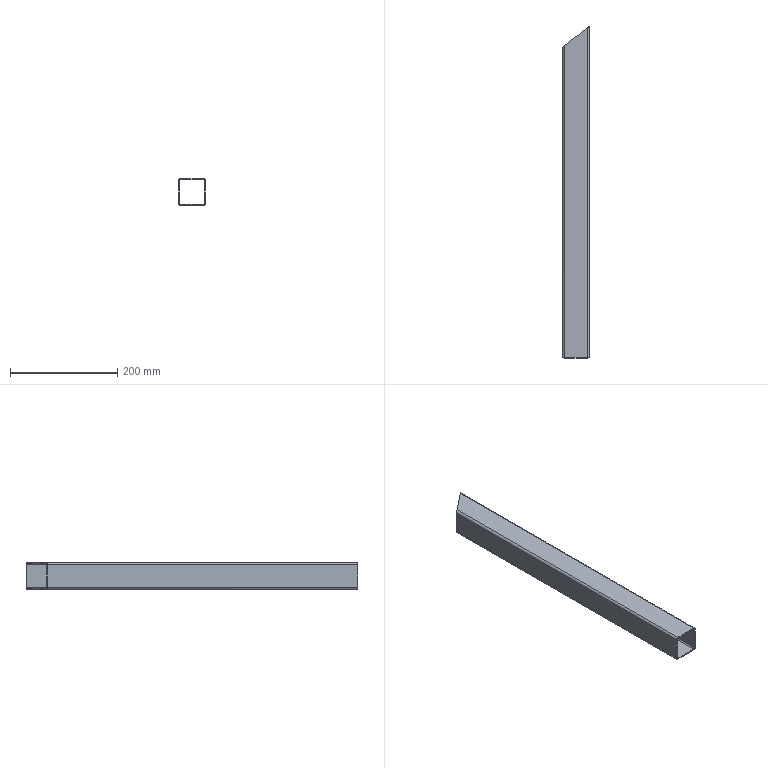Part | STEP file | Microwave Drying Flat Conveyor-CN2500x400-105-101_Default<Machining blank> | 1 solid | 18 faces | box 50 x 620 x 50 mm | volume 224219 mm3 | plane 10 | cylinder 8 | commonest cylinder face diameters 4 x4 8 x4
STEP:
#1=CARTESIAN_POINT('',(501.,0.,21.));
#2=VERTEX_POINT('',#1);
#3=CARTESIAN_POINT('',(501.,620.,21.));
#4=VERTEX_POINT('',#3);
#5=CARTESIAN_POINT('',(501.,0.,21.));
#6=DIRECTION('',(0.,1.,0.));
#7=VECTOR('',#6,1000.);
#8=LINE('',#5,#7);
#9=EDGE_CURVE('',#2,#4,#8,.T.);
#10=ORIENTED_EDGE('',*,*,#9,.T.);
#11=CARTESIAN_POINT('',(497.,616.8,25.));
#12=VERTEX_POINT('',#11);
#13=CARTESIAN_POINT('',(501.,620.,21.));
#14=CARTESIAN_POINT('',(501.,620.,23.343));
#15=CARTESIAN_POINT('',(499.343,618.675,25.));
#16=CARTESIAN_POINT('',(497.,616.8,25.));
#17=(BOUNDED_CURVE()B_SPLINE_CURVE(3,(#13,#14,#15,#16),.UNSPECIFIED.,.F.,.T.)B_SPLINE_CURVE_WITH_KNOTS((4,4),(0.,1.571),.UNSPECIFIED.)CURVE()GEOMETRIC_REPRESENTATION_ITEM()RATIONAL_B_SPLINE_CURVE((1.,0.8047,0.8047,1.))REPRESENTATION_ITEM(''));
#18=EDGE_CURVE('',#4,#12,#17,.T.);
#19=ORIENTED_EDGE('',*,*,#18,.T.);
#20=CARTESIAN_POINT('',(497.,0.,25.));
#21=VERTEX_POINT('',#20);
#22=CARTESIAN_POINT('',(497.,0.,25.));
#23=DIRECTION('',(0.,1.,0.));
#24=VECTOR('',#23,1000.);
#25=LINE('',#22,#24);
#26=EDGE_CURVE('',#21,#12,#25,.T.);
#27=ORIENTED_EDGE('',*,*,#26,.F.);
#28=CARTESIAN_POINT('',(497.,0.,21.));
#29=DIRECTION('',(0.,-1.,0.));
#30=DIRECTION('',(1.,0.,0.));
#31=AXIS2_PLACEMENT_3D('',#28,#29,#30);
#32=CIRCLE('',#31,4.);
#33=EDGE_CURVE('',#2,#21,#32,.T.);
#34=ORIENTED_EDGE('',*,*,#33,.F.);
#35=EDGE_LOOP('',(#10,#19,#27,#34));
#36=FACE_OUTER_BOUND('',#35,.T.);
#37=CARTESIAN_POINT('',(497.,0.,21.));
#38=DIRECTION('',(0.,1.,0.));
#39=DIRECTION('',(-1.,0.,0.));
#40=AXIS2_PLACEMENT_3D('',#37,#38,#39);
#41=CYLINDRICAL_SURFACE('',#40,4.);
#42=ADVANCED_FACE('',(#36),#41,.T.);
#43=ORIENTED_EDGE('',*,*,#26,.T.);
#44=CARTESIAN_POINT('',(455.,583.2,25.));
#45=VERTEX_POINT('',#44);
#46=CARTESIAN_POINT('',(501.,620.,25.));
#47=DIRECTION('',(0.7809,0.6247,0.));
#48=VECTOR('',#47,1000.);
#49=LINE('',#46,#48);
#50=EDGE_CURVE('',#45,#12,#49,.T.);
#51=ORIENTED_EDGE('',*,*,#50,.F.);
#52=CARTESIAN_POINT('',(455.,0.,25.));
#53=VERTEX_POINT('',#52);
#54=CARTESIAN_POINT('',(455.,0.,25.));
#55=DIRECTION('',(0.,1.,0.));
#56=VECTOR('',#55,1000.);
#57=LINE('',#54,#56);
#58=EDGE_CURVE('',#53,#45,#57,.T.);
#59=ORIENTED_EDGE('',*,*,#58,.F.);
#60=CARTESIAN_POINT('',(497.,0.,25.));
#61=DIRECTION('',(-1.,0.,0.));
#62=VECTOR('',#61,1000.);
#63=LINE('',#60,#62);
#64=EDGE_CURVE('',#21,#53,#63,.T.);
#65=ORIENTED_EDGE('',*,*,#64,.F.);
#66=EDGE_LOOP('',(#43,#51,#59,#65));
#67=FACE_OUTER_BOUND('',#66,.T.);
#68=CARTESIAN_POINT('',(497.,0.,25.));
#69=DIRECTION('',(0.,0.,-1.));
#70=DIRECTION('',(-1.,0.,0.));
#71=AXIS2_PLACEMENT_3D('',#68,#69,#70);
#72=PLANE('',#71);
#73=ADVANCED_FACE('',(#67),#72,.F.);
#74=ORIENTED_EDGE('',*,*,#58,.T.);
#75=CARTESIAN_POINT('',(451.,580.,21.));
#76=VERTEX_POINT('',#75);
#77=CARTESIAN_POINT('',(455.,583.2,25.));
#78=CARTESIAN_POINT('',(452.657,581.325,25.));
#79=CARTESIAN_POINT('',(451.,580.,23.343));
#80=CARTESIAN_POINT('',(451.,580.,21.));
#81=(BOUNDED_CURVE()B_SPLINE_CURVE(3,(#77,#78,#79,#80),.UNSPECIFIED.,.F.,.F.)B_SPLINE_CURVE_WITH_KNOTS((4,4),(1.571,3.142),.UNSPECIFIED.)CURVE()GEOMETRIC_REPRESENTATION_ITEM()RATIONAL_B_SPLINE_CURVE((1.,0.8047,0.8047,1.))REPRESENTATION_ITEM(''));
#82=EDGE_CURVE('',#45,#76,#81,.T.);
#83=ORIENTED_EDGE('',*,*,#82,.T.);
#84=CARTESIAN_POINT('',(451.,0.,21.));
#85=VERTEX_POINT('',#84);
#86=CARTESIAN_POINT('',(451.,0.,21.));
#87=DIRECTION('',(0.,1.,0.));
#88=VECTOR('',#87,1000.);
#89=LINE('',#86,#88);
#90=EDGE_CURVE('',#85,#76,#89,.T.);
#91=ORIENTED_EDGE('',*,*,#90,.F.);
#92=CARTESIAN_POINT('',(455.,0.,21.));
#93=DIRECTION('',(0.,-1.,0.));
#94=DIRECTION('',(1.,0.,0.));
#95=AXIS2_PLACEMENT_3D('',#92,#93,#94);
#96=CIRCLE('',#95,4.);
#97=EDGE_CURVE('',#53,#85,#96,.T.);
#98=ORIENTED_EDGE('',*,*,#97,.F.);
#99=EDGE_LOOP('',(#74,#83,#91,#98));
#100=FACE_OUTER_BOUND('',#99,.T.);
#101=CARTESIAN_POINT('',(455.,0.,21.));
#102=DIRECTION('',(0.,1.,0.));
#103=DIRECTION('',(-1.,0.,0.));
#104=AXIS2_PLACEMENT_3D('',#101,#102,#103);
#105=CYLINDRICAL_SURFACE('',#104,4.);
#106=ADVANCED_FACE('',(#100),#105,.T.);
#107=ORIENTED_EDGE('',*,*,#90,.T.);
#108=CARTESIAN_POINT('',(451.,580.,-21.));
#109=VERTEX_POINT('',#108);
#110=CARTESIAN_POINT('',(451.,580.,-25.));
#111=DIRECTION('',(0.,0.,1.));
#112=VECTOR('',#111,1000.);
#113=LINE('',#110,#112);
#114=EDGE_CURVE('',#109,#76,#113,.T.);
#115=ORIENTED_EDGE('',*,*,#114,.F.);
#116=CARTESIAN_POINT('',(451.,0.,-21.));
#117=VERTEX_POINT('',#116);
#118=CARTESIAN_POINT('',(451.,0.,-21.));
#119=DIRECTION('',(0.,1.,0.));
#120=VECTOR('',#119,1000.);
#121=LINE('',#118,#120);
#122=EDGE_CURVE('',#117,#109,#121,.T.);
#123=ORIENTED_EDGE('',*,*,#122,.F.);
#124=CARTESIAN_POINT('',(451.,0.,-21.));
#125=DIRECTION('',(0.,0.,-1.));
#126=VECTOR('',#125,1000.);
#127=LINE('',#124,#126);
#128=EDGE_CURVE('',#85,#117,#127,.T.);
#129=ORIENTED_EDGE('',*,*,#128,.F.);
#130=EDGE_LOOP('',(#107,#115,#123,#129));
#131=FACE_OUTER_BOUND('',#130,.T.);
#132=CARTESIAN_POINT('',(451.,0.,-21.));
#133=DIRECTION('',(1.,0.,0.));
#134=DIRECTION('',(0.,1.,0.));
#135=AXIS2_PLACEMENT_3D('',#132,#133,#134);
#136=PLANE('',#135);
#137=ADVANCED_FACE('',(#131),#136,.F.);
#138=ORIENTED_EDGE('',*,*,#122,.T.);
#139=CARTESIAN_POINT('',(455.,583.2,-25.));
#140=VERTEX_POINT('',#139);
#141=CARTESIAN_POINT('',(451.,580.,-21.));
#142=CARTESIAN_POINT('',(451.,580.,-23.343));
#143=CARTESIAN_POINT('',(452.657,581.325,-25.));
#144=CARTESIAN_POINT('',(455.,583.2,-25.));
#145=(BOUNDED_CURVE()B_SPLINE_CURVE(3,(#141,#142,#143,#144),.UNSPECIFIED.,.F.,.F.)B_SPLINE_CURVE_WITH_KNOTS((4,4),(3.142,4.712),.UNSPECIFIED.)CURVE()GEOMETRIC_REPRESENTATION_ITEM()RATIONAL_B_SPLINE_CURVE((1.,0.8047,0.8047,1.))REPRESENTATION_ITEM(''));
#146=EDGE_CURVE('',#109,#140,#145,.T.);
#147=ORIENTED_EDGE('',*,*,#146,.T.);
#148=CARTESIAN_POINT('',(455.,0.,-25.));
#149=VERTEX_POINT('',#148);
#150=CARTESIAN_POINT('',(455.,0.,-25.));
#151=DIRECTION('',(0.,1.,0.));
#152=VECTOR('',#151,1000.);
#153=LINE('',#150,#152);
#154=EDGE_CURVE('',#149,#140,#153,.T.);
#155=ORIENTED_EDGE('',*,*,#154,.F.);
#156=CARTESIAN_POINT('',(455.,0.,-21.));
#157=DIRECTION('',(0.,-1.,0.));
#158=DIRECTION('',(1.,0.,0.));
#159=AXIS2_PLACEMENT_3D('',#156,#157,#158);
#160=CIRCLE('',#159,4.);
#161=EDGE_CURVE('',#117,#149,#160,.T.);
#162=ORIENTED_EDGE('',*,*,#161,.F.);
#163=EDGE_LOOP('',(#138,#147,#155,#162));
#164=FACE_OUTER_BOUND('',#163,.T.);
#165=CARTESIAN_POINT('',(455.,0.,-21.));
#166=DIRECTION('',(0.,1.,0.));
#167=DIRECTION('',(-1.,0.,0.));
#168=AXIS2_PLACEMENT_3D('',#165,#166,#167);
#169=CYLINDRICAL_SURFACE('',#168,4.);
#170=ADVANCED_FACE('',(#164),#169,.T.);
#171=ORIENTED_EDGE('',*,*,#154,.T.);
#172=CARTESIAN_POINT('',(497.,616.8,-25.));
#173=VERTEX_POINT('',#172);
#174=CARTESIAN_POINT('',(501.,620.,-25.));
#175=DIRECTION('',(0.7809,0.6247,0.));
#176=VECTOR('',#175,1000.);
#177=LINE('',#174,#176);
#178=EDGE_CURVE('',#140,#173,#177,.T.);
#179=ORIENTED_EDGE('',*,*,#178,.T.);
#180=CARTESIAN_POINT('',(497.,0.,-25.));
#181=VERTEX_POINT('',#180);
#182=CARTESIAN_POINT('',(497.,0.,-25.));
#183=DIRECTION('',(0.,1.,0.));
#184=VECTOR('',#183,1000.);
#185=LINE('',#182,#184);
#186=EDGE_CURVE('',#181,#173,#185,.T.);
#187=ORIENTED_EDGE('',*,*,#186,.F.);
#188=CARTESIAN_POINT('',(455.,0.,-25.));
#189=DIRECTION('',(1.,0.,0.));
#190=VECTOR('',#189,1000.);
#191=LINE('',#188,#190);
#192=EDGE_CURVE('',#149,#181,#191,.T.);
#193=ORIENTED_EDGE('',*,*,#192,.F.);
#194=EDGE_LOOP('',(#171,#179,#187,#193));
#195=FACE_OUTER_BOUND('',#194,.T.);
#196=CARTESIAN_POINT('',(455.,0.,-25.));
#197=DIRECTION('',(0.,0.,1.));
#198=DIRECTION('',(1.,0.,0.));
#199=AXIS2_PLACEMENT_3D('',#196,#197,#198);
#200=PLANE('',#199);
#201=ADVANCED_FACE('',(#195),#200,.F.);
#202=ORIENTED_EDGE('',*,*,#186,.T.);
#203=CARTESIAN_POINT('',(501.,620.,-21.));
#204=VERTEX_POINT('',#203);
#205=CARTESIAN_POINT('',(497.,616.8,-25.));
#206=CARTESIAN_POINT('',(499.343,618.675,-25.));
#207=CARTESIAN_POINT('',(501.,620.,-23.343));
#208=CARTESIAN_POINT('',(501.,620.,-21.));
#209=(BOUNDED_CURVE()B_SPLINE_CURVE(3,(#205,#206,#207,#208),.UNSPECIFIED.,.F.,.T.)B_SPLINE_CURVE_WITH_KNOTS((4,4),(4.712,6.283),.UNSPECIFIED.)CURVE()GEOMETRIC_REPRESENTATION_ITEM()RATIONAL_B_SPLINE_CURVE((1.,0.8047,0.8047,1.))REPRESENTATION_ITEM(''));
#210=EDGE_CURVE('',#173,#204,#209,.T.);
#211=ORIENTED_EDGE('',*,*,#210,.T.);
#212=CARTESIAN_POINT('',(501.,0.,-21.));
#213=VERTEX_POINT('',#212);
#214=CARTESIAN_POINT('',(501.,0.,-21.));
#215=DIRECTION('',(0.,1.,0.));
#216=VECTOR('',#215,1000.);
#217=LINE('',#214,#216);
#218=EDGE_CURVE('',#213,#204,#217,.T.);
#219=ORIENTED_EDGE('',*,*,#218,.F.);
#220=CARTESIAN_POINT('',(497.,0.,-21.));
#221=DIRECTION('',(0.,-1.,0.));
#222=DIRECTION('',(1.,0.,0.));
#223=AXIS2_PLACEMENT_3D('',#220,#221,#222);
#224=CIRCLE('',#223,4.);
#225=EDGE_CURVE('',#181,#213,#224,.T.);
#226=ORIENTED_EDGE('',*,*,#225,.F.);
#227=EDGE_LOOP('',(#202,#211,#219,#226));
#228=FACE_OUTER_BOUND('',#227,.T.);
#229=CARTESIAN_POINT('',(497.,0.,-21.));
#230=DIRECTION('',(0.,1.,0.));
#231=DIRECTION('',(-1.,0.,0.));
#232=AXIS2_PLACEMENT_3D('',#229,#230,#231);
#233=CYLINDRICAL_SURFACE('',#232,4.);
#234=ADVANCED_FACE('',(#228),#233,.T.);
#235=CARTESIAN_POINT('',(455.,583.2,23.));
#236=VERTEX_POINT('',#235);
#237=CARTESIAN_POINT('',(453.,581.6,21.));
#238=VERTEX_POINT('',#237);
#239=CARTESIAN_POINT('',(455.,583.2,23.));
#240=CARTESIAN_POINT('',(453.828,582.263,23.));
#241=CARTESIAN_POINT('',(453.,581.6,22.172));
#242=CARTESIAN_POINT('',(453.,581.6,21.));
#243=(BOUNDED_CURVE()B_SPLINE_CURVE(3,(#239,#240,#241,#242),.UNSPECIFIED.,.F.,.F.)B_SPLINE_CURVE_WITH_KNOTS((4,4),(1.571,3.142),.UNSPECIFIED.)CURVE()GEOMETRIC_REPRESENTATION_ITEM()RATIONAL_B_SPLINE_CURVE((1.,0.8047,0.8047,1.))REPRESENTATION_ITEM(''));
#244=EDGE_CURVE('',#236,#238,#243,.T.);
#245=ORIENTED_EDGE('',*,*,#244,.F.);
#246=CARTESIAN_POINT('',(455.,0.,23.));
#247=VERTEX_POINT('',#246);
#248=CARTESIAN_POINT('',(455.,0.,23.));
#249=DIRECTION('',(0.,1.,0.));
#250=VECTOR('',#249,1000.);
#251=LINE('',#248,#250);
#252=EDGE_CURVE('',#247,#236,#251,.T.);
#253=ORIENTED_EDGE('',*,*,#252,.F.);
#254=CARTESIAN_POINT('',(453.,0.,21.));
#255=VERTEX_POINT('',#254);
#256=CARTESIAN_POINT('',(455.,0.,21.));
#257=DIRECTION('',(0.,-1.,0.));
#258=DIRECTION('',(1.,0.,0.));
#259=AXIS2_PLACEMENT_3D('',#256,#257,#258);
#260=CIRCLE('',#259,2.);
#261=EDGE_CURVE('',#247,#255,#260,.T.);
#262=ORIENTED_EDGE('',*,*,#261,.T.);
#263=CARTESIAN_POINT('',(453.,0.,21.));
#264=DIRECTION('',(0.,1.,0.));
#265=VECTOR('',#264,1000.);
#266=LINE('',#263,#265);
#267=EDGE_CURVE('',#255,#238,#266,.T.);
#268=ORIENTED_EDGE('',*,*,#267,.T.);
#269=EDGE_LOOP('',(#245,#253,#262,#268));
#270=FACE_OUTER_BOUND('',#269,.T.);
#271=CARTESIAN_POINT('',(455.,0.,21.));
#272=DIRECTION('',(0.,1.,0.));
#273=DIRECTION('',(-1.,0.,0.));
#274=AXIS2_PLACEMENT_3D('',#271,#272,#273);
#275=CYLINDRICAL_SURFACE('',#274,2.);
#276=ADVANCED_FACE('',(#270),#275,.F.);
#277=CARTESIAN_POINT('',(497.,616.8,23.));
#278=VERTEX_POINT('',#277);
#279=CARTESIAN_POINT('',(196.122,376.098,23.));
#280=DIRECTION('',(-0.7809,-0.6247,0.));
#281=VECTOR('',#280,1000.);
#282=LINE('',#279,#281);
#283=EDGE_CURVE('',#278,#236,#282,.T.);
#284=ORIENTED_EDGE('',*,*,#283,.F.);
#285=CARTESIAN_POINT('',(497.,0.,23.));
#286=VERTEX_POINT('',#285);
#287=CARTESIAN_POINT('',(497.,0.,23.));
#288=DIRECTION('',(0.,1.,0.));
#289=VECTOR('',#288,1000.);
#290=LINE('',#287,#289);
#291=EDGE_CURVE('',#286,#278,#290,.T.);
#292=ORIENTED_EDGE('',*,*,#291,.F.);
#293=CARTESIAN_POINT('',(497.,0.,23.));
#294=DIRECTION('',(-1.,0.,0.));
#295=VECTOR('',#294,1000.);
#296=LINE('',#293,#295);
#297=EDGE_CURVE('',#286,#247,#296,.T.);
#298=ORIENTED_EDGE('',*,*,#297,.T.);
#299=ORIENTED_EDGE('',*,*,#252,.T.);
#300=EDGE_LOOP('',(#284,#292,#298,#299));
#301=FACE_OUTER_BOUND('',#300,.T.);
#302=CARTESIAN_POINT('',(497.,0.,23.));
#303=DIRECTION('',(0.,0.,-1.));
#304=DIRECTION('',(-1.,0.,0.));
#305=AXIS2_PLACEMENT_3D('',#302,#303,#304);
#306=PLANE('',#305);
#307=ADVANCED_FACE('',(#301),#306,.T.);
#308=CARTESIAN_POINT('',(499.,618.4,21.));
#309=VERTEX_POINT('',#308);
#310=CARTESIAN_POINT('',(499.,618.4,21.));
#311=CARTESIAN_POINT('',(499.,618.4,22.172));
#312=CARTESIAN_POINT('',(498.172,617.737,23.));
#313=CARTESIAN_POINT('',(497.,616.8,23.));
#314=(BOUNDED_CURVE()B_SPLINE_CURVE(3,(#310,#311,#312,#313),.UNSPECIFIED.,.F.,.T.)B_SPLINE_CURVE_WITH_KNOTS((4,4),(0.,1.571),.UNSPECIFIED.)CURVE()GEOMETRIC_REPRESENTATION_ITEM()RATIONAL_B_SPLINE_CURVE((1.,0.8047,0.8047,1.))REPRESENTATION_ITEM(''));
#315=EDGE_CURVE('',#309,#278,#314,.T.);
#316=ORIENTED_EDGE('',*,*,#315,.F.);
#317=CARTESIAN_POINT('',(499.,0.,21.));
#318=VERTEX_POINT('',#317);
#319=CARTESIAN_POINT('',(499.,0.,21.));
#320=DIRECTION('',(0.,1.,0.));
#321=VECTOR('',#320,1000.);
#322=LINE('',#319,#321);
#323=EDGE_CURVE('',#318,#309,#322,.T.);
#324=ORIENTED_EDGE('',*,*,#323,.F.);
#325=CARTESIAN_POINT('',(497.,0.,21.));
#326=DIRECTION('',(0.,-1.,0.));
#327=DIRECTION('',(1.,0.,0.));
#328=AXIS2_PLACEMENT_3D('',#325,#326,#327);
#329=CIRCLE('',#328,2.);
#330=EDGE_CURVE('',#318,#286,#329,.T.);
#331=ORIENTED_EDGE('',*,*,#330,.T.);
#332=ORIENTED_EDGE('',*,*,#291,.T.);
#333=EDGE_LOOP('',(#316,#324,#331,#332));
#334=FACE_OUTER_BOUND('',#333,.T.);
#335=CARTESIAN_POINT('',(497.,0.,21.));
#336=DIRECTION('',(0.,1.,0.));
#337=DIRECTION('',(-1.,0.,0.));
#338=AXIS2_PLACEMENT_3D('',#335,#336,#337);
#339=CYLINDRICAL_SURFACE('',#338,2.);
#340=ADVANCED_FACE('',(#334),#339,.F.);
#341=CARTESIAN_POINT('',(499.,618.4,-21.));
#342=VERTEX_POINT('',#341);
#343=CARTESIAN_POINT('',(499.,618.4,21.));
#344=DIRECTION('',(0.,0.,1.));
#345=VECTOR('',#344,1000.);
#346=LINE('',#343,#345);
#347=EDGE_CURVE('',#342,#309,#346,.T.);
#348=ORIENTED_EDGE('',*,*,#347,.F.);
#349=CARTESIAN_POINT('',(499.,0.,-21.));
#350=VERTEX_POINT('',#349);
#351=CARTESIAN_POINT('',(499.,0.,-21.));
#352=DIRECTION('',(0.,1.,0.));
#353=VECTOR('',#352,1000.);
#354=LINE('',#351,#353);
#355=EDGE_CURVE('',#350,#342,#354,.T.);
#356=ORIENTED_EDGE('',*,*,#355,.F.);
#357=CARTESIAN_POINT('',(499.,0.,21.));
#358=DIRECTION('',(0.,0.,1.));
#359=VECTOR('',#358,1000.);
#360=LINE('',#357,#359);
#361=EDGE_CURVE('',#350,#318,#360,.T.);
#362=ORIENTED_EDGE('',*,*,#361,.T.);
#363=ORIENTED_EDGE('',*,*,#323,.T.);
#364=EDGE_LOOP('',(#348,#356,#362,#363));
#365=FACE_OUTER_BOUND('',#364,.T.);
#366=CARTESIAN_POINT('',(499.,0.,21.));
#367=DIRECTION('',(-1.,0.,0.));
#368=DIRECTION('',(0.,-1.,0.));
#369=AXIS2_PLACEMENT_3D('',#366,#367,#368);
#370=PLANE('',#369);
#371=ADVANCED_FACE('',(#365),#370,.T.);
#372=CARTESIAN_POINT('',(497.,616.8,-23.));
#373=VERTEX_POINT('',#372);
#374=CARTESIAN_POINT('',(497.,616.8,-23.));
#375=CARTESIAN_POINT('',(498.172,617.737,-23.));
#376=CARTESIAN_POINT('',(499.,618.4,-22.172));
#377=CARTESIAN_POINT('',(499.,618.4,-21.));
#378=(BOUNDED_CURVE()B_SPLINE_CURVE(3,(#374,#375,#376,#377),.UNSPECIFIED.,.F.,.F.)B_SPLINE_CURVE_WITH_KNOTS((4,4),(4.712,6.283),.UNSPECIFIED.)CURVE()GEOMETRIC_REPRESENTATION_ITEM()RATIONAL_B_SPLINE_CURVE((1.,0.8047,0.8047,1.))REPRESENTATION_ITEM(''));
#379=EDGE_CURVE('',#373,#342,#378,.T.);
#380=ORIENTED_EDGE('',*,*,#379,.F.);
#381=CARTESIAN_POINT('',(497.,0.,-23.));
#382=VERTEX_POINT('',#381);
#383=CARTESIAN_POINT('',(497.,0.,-23.));
#384=DIRECTION('',(0.,1.,0.));
#385=VECTOR('',#384,1000.);
#386=LINE('',#383,#385);
#387=EDGE_CURVE('',#382,#373,#386,.T.);
#388=ORIENTED_EDGE('',*,*,#387,.F.);
#389=CARTESIAN_POINT('',(497.,0.,-21.));
#390=DIRECTION('',(0.,-1.,0.));
#391=DIRECTION('',(1.,0.,0.));
#392=AXIS2_PLACEMENT_3D('',#389,#390,#391);
#393=CIRCLE('',#392,2.);
#394=EDGE_CURVE('',#382,#350,#393,.T.);
#395=ORIENTED_EDGE('',*,*,#394,.T.);
#396=ORIENTED_EDGE('',*,*,#355,.T.);
#397=EDGE_LOOP('',(#380,#388,#395,#396));
#398=FACE_OUTER_BOUND('',#397,.T.);
#399=CARTESIAN_POINT('',(497.,0.,-21.));
#400=DIRECTION('',(0.,1.,0.));
#401=DIRECTION('',(-1.,0.,0.));
#402=AXIS2_PLACEMENT_3D('',#399,#400,#401);
#403=CYLINDRICAL_SURFACE('',#402,2.);
#404=ADVANCED_FACE('',(#398),#403,.F.);
#405=CARTESIAN_POINT('',(455.,583.2,-23.));
#406=VERTEX_POINT('',#405);
#407=CARTESIAN_POINT('',(170.512,355.61,-23.));
#408=DIRECTION('',(0.7809,0.6247,0.));
#409=VECTOR('',#408,1000.);
#410=LINE('',#407,#409);
#411=EDGE_CURVE('',#406,#373,#410,.T.);
#412=ORIENTED_EDGE('',*,*,#411,.F.);
#413=CARTESIAN_POINT('',(455.,0.,-23.));
#414=VERTEX_POINT('',#413);
#415=CARTESIAN_POINT('',(455.,0.,-23.));
#416=DIRECTION('',(0.,1.,0.));
#417=VECTOR('',#416,1000.);
#418=LINE('',#415,#417);
#419=EDGE_CURVE('',#414,#406,#418,.T.);
#420=ORIENTED_EDGE('',*,*,#419,.F.);
#421=CARTESIAN_POINT('',(455.,0.,-23.));
#422=DIRECTION('',(1.,0.,0.));
#423=VECTOR('',#422,1000.);
#424=LINE('',#421,#423);
#425=EDGE_CURVE('',#414,#382,#424,.T.);
#426=ORIENTED_EDGE('',*,*,#425,.T.);
#427=ORIENTED_EDGE('',*,*,#387,.T.);
#428=EDGE_LOOP('',(#412,#420,#426,#427));
#429=FACE_OUTER_BOUND('',#428,.T.);
#430=CARTESIAN_POINT('',(455.,0.,-23.));
#431=DIRECTION('',(0.,0.,1.));
#432=DIRECTION('',(1.,0.,0.));
#433=AXIS2_PLACEMENT_3D('',#430,#431,#432);
#434=PLANE('',#433);
#435=ADVANCED_FACE('',(#429),#434,.T.);
#436=CARTESIAN_POINT('',(453.,581.6,-21.));
#437=VERTEX_POINT('',#436);
#438=CARTESIAN_POINT('',(453.,581.6,-21.));
#439=CARTESIAN_POINT('',(453.,581.6,-22.172));
#440=CARTESIAN_POINT('',(453.828,582.263,-23.));
#441=CARTESIAN_POINT('',(455.,583.2,-23.));
#442=(BOUNDED_CURVE()B_SPLINE_CURVE(3,(#438,#439,#440,#441),.UNSPECIFIED.,.F.,.T.)B_SPLINE_CURVE_WITH_KNOTS((4,4),(3.142,4.712),.UNSPECIFIED.)CURVE()GEOMETRIC_REPRESENTATION_ITEM()RATIONAL_B_SPLINE_CURVE((1.,0.8047,0.8047,1.))REPRESENTATION_ITEM(''));
#443=EDGE_CURVE('',#437,#406,#442,.T.);
#444=ORIENTED_EDGE('',*,*,#443,.F.);
#445=CARTESIAN_POINT('',(453.,0.,-21.));
#446=VERTEX_POINT('',#445);
#447=CARTESIAN_POINT('',(453.,0.,-21.));
#448=DIRECTION('',(0.,1.,0.));
#449=VECTOR('',#448,1000.);
#450=LINE('',#447,#449);
#451=EDGE_CURVE('',#446,#437,#450,.T.);
#452=ORIENTED_EDGE('',*,*,#451,.F.);
#453=CARTESIAN_POINT('',(455.,0.,-21.));
#454=DIRECTION('',(0.,-1.,0.));
#455=DIRECTION('',(1.,0.,0.));
#456=AXIS2_PLACEMENT_3D('',#453,#454,#455);
#457=CIRCLE('',#456,2.);
#458=EDGE_CURVE('',#446,#414,#457,.T.);
#459=ORIENTED_EDGE('',*,*,#458,.T.);
#460=ORIENTED_EDGE('',*,*,#419,.T.);
#461=EDGE_LOOP('',(#444,#452,#459,#460));
#462=FACE_OUTER_BOUND('',#461,.T.);
#463=CARTESIAN_POINT('',(455.,0.,-21.));
#464=DIRECTION('',(0.,1.,0.));
#465=DIRECTION('',(-1.,0.,0.));
#466=AXIS2_PLACEMENT_3D('',#463,#464,#465);
#467=CYLINDRICAL_SURFACE('',#466,2.);
#468=ADVANCED_FACE('',(#462),#467,.F.);
#469=CARTESIAN_POINT('',(453.,581.6,-21.));
#470=DIRECTION('',(0.,0.,-1.));
#471=VECTOR('',#470,1000.);
#472=LINE('',#469,#471);
#473=EDGE_CURVE('',#238,#437,#472,.T.);
#474=ORIENTED_EDGE('',*,*,#473,.F.);
#475=ORIENTED_EDGE('',*,*,#267,.F.);
#476=CARTESIAN_POINT('',(453.,0.,-21.));
#477=DIRECTION('',(0.,0.,-1.));
#478=VECTOR('',#477,1000.);
#479=LINE('',#476,#478);
#480=EDGE_CURVE('',#255,#446,#479,.T.);
#481=ORIENTED_EDGE('',*,*,#480,.T.);
#482=ORIENTED_EDGE('',*,*,#451,.T.);
#483=EDGE_LOOP('',(#474,#475,#481,#482));
#484=FACE_OUTER_BOUND('',#483,.T.);
#485=CARTESIAN_POINT('',(453.,0.,-21.));
#486=DIRECTION('',(1.,0.,0.));
#487=DIRECTION('',(0.,1.,0.));
#488=AXIS2_PLACEMENT_3D('',#485,#486,#487);
#489=PLANE('',#488);
#490=ADVANCED_FACE('',(#484),#489,.T.);
#491=CARTESIAN_POINT('',(501.,620.,21.));
#492=DIRECTION('',(0.,0.,1.));
#493=VECTOR('',#492,1000.);
#494=LINE('',#491,#493);
#495=EDGE_CURVE('',#204,#4,#494,.T.);
#496=ORIENTED_EDGE('',*,*,#495,.T.);
#497=ORIENTED_EDGE('',*,*,#9,.F.);
#498=CARTESIAN_POINT('',(501.,0.,21.));
#499=DIRECTION('',(0.,0.,1.));
#500=VECTOR('',#499,1000.);
#501=LINE('',#498,#500);
#502=EDGE_CURVE('',#213,#2,#501,.T.);
#503=ORIENTED_EDGE('',*,*,#502,.F.);
#504=ORIENTED_EDGE('',*,*,#218,.T.);
#505=EDGE_LOOP('',(#496,#497,#503,#504));
#506=FACE_OUTER_BOUND('',#505,.T.);
#507=CARTESIAN_POINT('',(501.,0.,21.));
#508=DIRECTION('',(-1.,0.,0.));
#509=DIRECTION('',(0.,-1.,0.));
#510=AXIS2_PLACEMENT_3D('',#507,#508,#509);
#511=PLANE('',#510);
#512=ADVANCED_FACE('',(#506),#511,.F.);
#513=ORIENTED_EDGE('',*,*,#261,.F.);
#514=ORIENTED_EDGE('',*,*,#297,.F.);
#515=ORIENTED_EDGE('',*,*,#330,.F.);
#516=ORIENTED_EDGE('',*,*,#361,.F.);
#517=ORIENTED_EDGE('',*,*,#394,.F.);
#518=ORIENTED_EDGE('',*,*,#425,.F.);
#519=ORIENTED_EDGE('',*,*,#458,.F.);
#520=ORIENTED_EDGE('',*,*,#480,.F.);
#521=EDGE_LOOP('',(#513,#514,#515,#516,#517,#518,#519,#520));
#522=FACE_BOUND('',#521,.T.);
#523=ORIENTED_EDGE('',*,*,#33,.T.);
#524=ORIENTED_EDGE('',*,*,#64,.T.);
#525=ORIENTED_EDGE('',*,*,#97,.T.);
#526=ORIENTED_EDGE('',*,*,#128,.T.);
#527=ORIENTED_EDGE('',*,*,#161,.T.);
#528=ORIENTED_EDGE('',*,*,#192,.T.);
#529=ORIENTED_EDGE('',*,*,#225,.T.);
#530=ORIENTED_EDGE('',*,*,#502,.T.);
#531=EDGE_LOOP('',(#523,#524,#525,#526,#527,#528,#529,#530));
#532=FACE_OUTER_BOUND('',#531,.T.);
#533=CARTESIAN_POINT('',(497.,0.,21.));
#534=DIRECTION('',(0.,-1.,0.));
#535=DIRECTION('',(1.,0.,0.));
#536=AXIS2_PLACEMENT_3D('',#533,#534,#535);
#537=PLANE('',#536);
#538=ADVANCED_FACE('',(#522,#532),#537,.T.);
#539=ORIENTED_EDGE('',*,*,#244,.T.);
#540=ORIENTED_EDGE('',*,*,#473,.T.);
#541=ORIENTED_EDGE('',*,*,#443,.T.);
#542=ORIENTED_EDGE('',*,*,#411,.T.);
#543=ORIENTED_EDGE('',*,*,#379,.T.);
#544=ORIENTED_EDGE('',*,*,#347,.T.);
#545=ORIENTED_EDGE('',*,*,#315,.T.);
#546=ORIENTED_EDGE('',*,*,#283,.T.);
#547=EDGE_LOOP('',(#539,#540,#541,#542,#543,#544,#545,#546));
#548=FACE_BOUND('',#547,.T.);
#549=ORIENTED_EDGE('',*,*,#495,.F.);
#550=ORIENTED_EDGE('',*,*,#210,.F.);
#551=ORIENTED_EDGE('',*,*,#178,.F.);
#552=ORIENTED_EDGE('',*,*,#146,.F.);
#553=ORIENTED_EDGE('',*,*,#114,.T.);
#554=ORIENTED_EDGE('',*,*,#82,.F.);
#555=ORIENTED_EDGE('',*,*,#50,.T.);
#556=ORIENTED_EDGE('',*,*,#18,.F.);
#557=EDGE_LOOP('',(#549,#550,#551,#552,#553,#554,#555,#556));
#558=FACE_OUTER_BOUND('',#557,.T.);
#559=CARTESIAN_POINT('',(501.,620.,-25.));
#560=DIRECTION('',(0.6247,-0.7809,0.));
#561=DIRECTION('',(0.7809,0.6247,0.));
#562=AXIS2_PLACEMENT_3D('',#559,#560,#561);
#563=PLANE('',#562);
#564=ADVANCED_FACE('',(#548,#558),#563,.F.);
#565=CLOSED_SHELL('',(#42,#73,#106,#137,#170,#201,#234,#276,#307,#340,#371,#404,#435,#468,#490,#512,#538,#564));
#566=MANIFOLD_SOLID_BREP('',#565);
#567=CARTESIAN_POINT('',(0.,0.,0.));
#568=DIRECTION('',(0.,0.,1.));
#569=DIRECTION('',(1.,0.,0.));
#570=AXIS2_PLACEMENT_3D('',#567,#568,#569);
#571=(LENGTH_UNIT()NAMED_UNIT(*)SI_UNIT(.MILLI.,.METRE.));
#572=UNCERTAINTY_MEASURE_WITH_UNIT(LENGTH_MEASURE(0.00001),#571,'','');
#573=(NAMED_UNIT(*)PLANE_ANGLE_UNIT()SI_UNIT($,.RADIAN.));
#574=(NAMED_UNIT(*)SI_UNIT($,.STERADIAN.)SOLID_ANGLE_UNIT());
#575=(GEOMETRIC_REPRESENTATION_CONTEXT(3)GLOBAL_UNCERTAINTY_ASSIGNED_CONTEXT((#572))GLOBAL_UNIT_ASSIGNED_CONTEXT((#571,#573,#574))REPRESENTATION_CONTEXT('',''));
#576=ADVANCED_BREP_SHAPE_REPRESENTATION('',(#566,#570),#575);